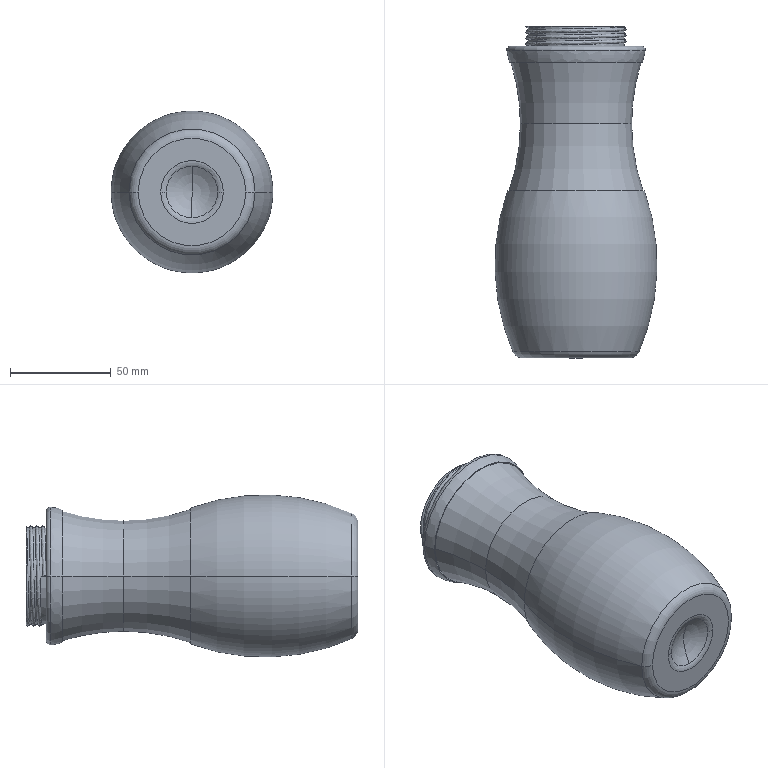Part | SolidWorks | features ICE 3, BaseBody 2, Fillet 2, Blend 1, CombineBodies 1, DeleteBody 1, Helix 1, OffsetRefSurface 1, RevCut 1, Revolution 1, Sculpt 1, Shell 1, Sweep 1, Thicken 1 | 1 solid | 56 faces | volume 63029 mm3 | torus 32 | cylinder 12 | plane 7 | cone 4 | spline 1 | commonest cylinder face diameters 48 x8 44 x2 46 x2